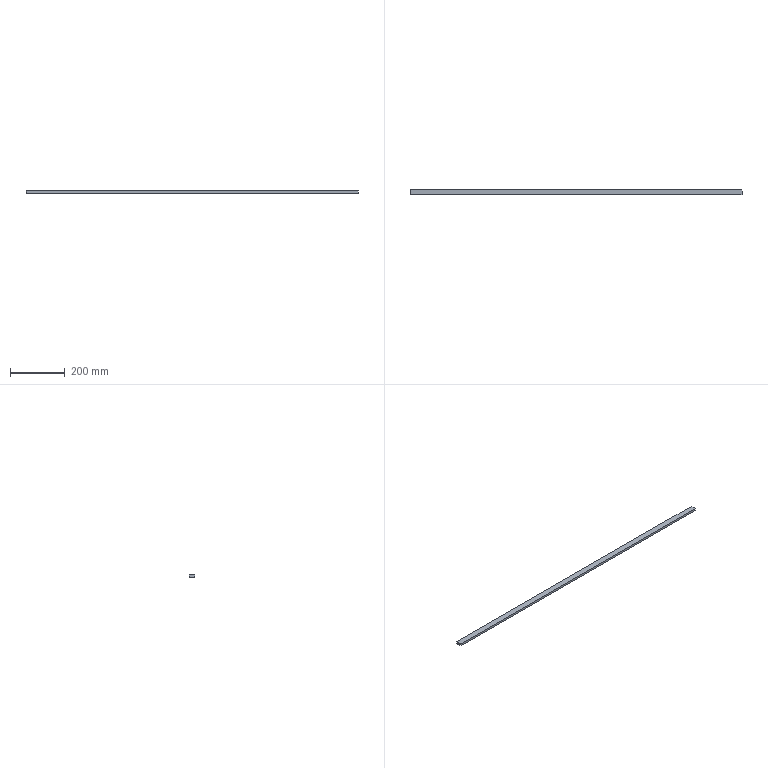Part | SolidWorks | features BaseBody 1 | 1 solid | 9 faces | box 1210 x 20 x 8 mm | volume 193263 mm3 | plane 9
STEP:
#1=CARTESIAN_POINT('',(605.05,-10.,-4.));
#2=VERTEX_POINT('',#1);
#3=CARTESIAN_POINT('',(-602.31,-10.,-4.));
#4=VERTEX_POINT('',#3);
#5=CARTESIAN_POINT('',(1.37,-10.,-4.));
#6=DIRECTION('',(-1.,0.,0.));
#7=VECTOR('',#6,1000.);
#8=LINE('',#5,#7);
#9=EDGE_CURVE('',#2,#4,#8,.T.);
#10=ORIENTED_EDGE('',*,*,#9,.F.);
#11=CARTESIAN_POINT('',(605.05,-10.,4.));
#12=VERTEX_POINT('',#11);
#13=CARTESIAN_POINT('',(605.05,-10.,0.));
#14=DIRECTION('',(0.,0.,-1.));
#15=VECTOR('',#14,1000.);
#16=LINE('',#13,#15);
#17=EDGE_CURVE('',#12,#2,#16,.T.);
#18=ORIENTED_EDGE('',*,*,#17,.F.);
#19=CARTESIAN_POINT('',(-602.31,-10.,4.));
#20=VERTEX_POINT('',#19);
#21=CARTESIAN_POINT('',(1.37,-10.,4.));
#22=DIRECTION('',(1.,0.,0.));
#23=VECTOR('',#22,1000.);
#24=LINE('',#21,#23);
#25=EDGE_CURVE('',#20,#12,#24,.T.);
#26=ORIENTED_EDGE('',*,*,#25,.F.);
#27=CARTESIAN_POINT('',(-602.31,-10.,0.));
#28=DIRECTION('',(0.,0.,1.));
#29=VECTOR('',#28,1000.);
#30=LINE('',#27,#29);
#31=EDGE_CURVE('',#4,#20,#30,.T.);
#32=ORIENTED_EDGE('',*,*,#31,.F.);
#33=EDGE_LOOP('',(#10,#18,#26,#32));
#34=FACE_OUTER_BOUND('',#33,.T.);
#35=CARTESIAN_POINT('',(605.05,-10.,-4.));
#36=DIRECTION('',(0.,1.,0.));
#37=DIRECTION('',(-1.,0.,0.));
#38=AXIS2_PLACEMENT_3D('',#35,#36,#37);
#39=PLANE('',#38);
#40=ADVANCED_FACE('',(#34),#39,.F.);
#41=CARTESIAN_POINT('',(-605.05,10.,4.));
#42=VERTEX_POINT('',#41);
#43=CARTESIAN_POINT('',(-605.05,10.,-4.));
#44=VERTEX_POINT('',#43);
#45=CARTESIAN_POINT('',(-605.05,10.,0.));
#46=DIRECTION('',(0.,0.,-1.));
#47=VECTOR('',#46,1000.);
#48=LINE('',#45,#47);
#49=EDGE_CURVE('',#42,#44,#48,.T.);
#50=ORIENTED_EDGE('',*,*,#49,.T.);
#51=CARTESIAN_POINT('',(-603.68,0.,-4.));
#52=DIRECTION('',(0.1357,-0.9907,0.));
#53=VECTOR('',#52,1000.);
#54=LINE('',#51,#53);
#55=EDGE_CURVE('',#44,#4,#54,.T.);
#56=ORIENTED_EDGE('',*,*,#55,.T.);
#57=ORIENTED_EDGE('',*,*,#31,.T.);
#58=CARTESIAN_POINT('',(-603.68,0.,4.));
#59=DIRECTION('',(-0.1357,0.9907,0.));
#60=VECTOR('',#59,1000.);
#61=LINE('',#58,#60);
#62=EDGE_CURVE('',#20,#42,#61,.T.);
#63=ORIENTED_EDGE('',*,*,#62,.T.);
#64=EDGE_LOOP('',(#50,#56,#57,#63));
#65=FACE_OUTER_BOUND('',#64,.T.);
#66=CARTESIAN_POINT('',(-605.05,10.,-4.));
#67=DIRECTION('',(-0.9907,-0.1357,0.));
#68=DIRECTION('',(0.1357,-0.9907,0.));
#69=AXIS2_PLACEMENT_3D('',#66,#67,#68);
#70=PLANE('',#69);
#71=ADVANCED_FACE('',(#65),#70,.T.);
#72=CARTESIAN_POINT('',(592.561,10.,-4.));
#73=VERTEX_POINT('',#72);
#74=CARTESIAN_POINT('',(592.561,8.975,-4.));
#75=VERTEX_POINT('',#74);
#76=CARTESIAN_POINT('',(592.561,9.488,-4.));
#77=DIRECTION('',(0.,-1.,0.));
#78=VECTOR('',#77,1000.);
#79=LINE('',#76,#78);
#80=EDGE_CURVE('',#73,#75,#79,.T.);
#81=ORIENTED_EDGE('',*,*,#80,.T.);
#82=CARTESIAN_POINT('',(603.97,8.975,-4.));
#83=VERTEX_POINT('',#82);
#84=CARTESIAN_POINT('',(0.,8.975,-4.));
#85=DIRECTION('',(1.,0.,0.));
#86=VECTOR('',#85,1000.);
#87=LINE('',#84,#86);
#88=EDGE_CURVE('',#75,#83,#87,.T.);
#89=ORIENTED_EDGE('',*,*,#88,.T.);
#90=CARTESIAN_POINT('',(605.05,1.773,-4.));
#91=VERTEX_POINT('',#90);
#92=CARTESIAN_POINT('',(603.97,8.975,-4.));
#93=DIRECTION('',(0.1483,-0.9889,0.));
#94=VECTOR('',#93,1000.);
#95=LINE('',#92,#94);
#96=EDGE_CURVE('',#83,#91,#95,.T.);
#97=ORIENTED_EDGE('',*,*,#96,.T.);
#98=CARTESIAN_POINT('',(605.05,0.,-4.));
#99=DIRECTION('',(0.,-1.,0.));
#100=VECTOR('',#99,1000.);
#101=LINE('',#98,#100);
#102=EDGE_CURVE('',#91,#2,#101,.T.);
#103=ORIENTED_EDGE('',*,*,#102,.T.);
#104=ORIENTED_EDGE('',*,*,#9,.T.);
#105=ORIENTED_EDGE('',*,*,#55,.F.);
#106=CARTESIAN_POINT('',(0.,10.,-4.));
#107=DIRECTION('',(1.,0.,0.));
#108=VECTOR('',#107,1000.);
#109=LINE('',#106,#108);
#110=EDGE_CURVE('',#44,#73,#109,.T.);
#111=ORIENTED_EDGE('',*,*,#110,.T.);
#112=EDGE_LOOP('',(#81,#89,#97,#103,#104,#105,#111));
#113=FACE_OUTER_BOUND('',#112,.T.);
#114=CARTESIAN_POINT('',(605.05,-10.,-4.));
#115=DIRECTION('',(0.,0.,-1.));
#116=DIRECTION('',(-1.,0.,0.));
#117=AXIS2_PLACEMENT_3D('',#114,#115,#116);
#118=PLANE('',#117);
#119=ADVANCED_FACE('',(#113),#118,.T.);
#120=CARTESIAN_POINT('',(605.05,1.773,4.));
#121=VERTEX_POINT('',#120);
#122=CARTESIAN_POINT('',(605.05,1.773,0.));
#123=DIRECTION('',(0.,0.,-1.));
#124=VECTOR('',#123,1000.);
#125=LINE('',#122,#124);
#126=EDGE_CURVE('',#121,#91,#125,.T.);
#127=ORIENTED_EDGE('',*,*,#126,.F.);
#128=CARTESIAN_POINT('',(605.05,-4.114,4.));
#129=DIRECTION('',(0.,1.,0.));
#130=VECTOR('',#129,1000.);
#131=LINE('',#128,#130);
#132=EDGE_CURVE('',#12,#121,#131,.T.);
#133=ORIENTED_EDGE('',*,*,#132,.F.);
#134=ORIENTED_EDGE('',*,*,#17,.T.);
#135=ORIENTED_EDGE('',*,*,#102,.F.);
#136=EDGE_LOOP('',(#127,#133,#134,#135));
#137=FACE_OUTER_BOUND('',#136,.T.);
#138=CARTESIAN_POINT('',(605.05,-10.,-4.));
#139=DIRECTION('',(-1.,0.,0.));
#140=DIRECTION('',(0.,0.,1.));
#141=AXIS2_PLACEMENT_3D('',#138,#139,#140);
#142=PLANE('',#141);
#143=ADVANCED_FACE('',(#137),#142,.F.);
#144=CARTESIAN_POINT('',(603.97,8.975,4.));
#145=VERTEX_POINT('',#144);
#146=CARTESIAN_POINT('',(603.97,8.975,4.));
#147=DIRECTION('',(0.1483,-0.9889,0.));
#148=VECTOR('',#147,1000.);
#149=LINE('',#146,#148);
#150=EDGE_CURVE('',#145,#121,#149,.T.);
#151=ORIENTED_EDGE('',*,*,#150,.F.);
#152=CARTESIAN_POINT('',(592.561,8.975,4.));
#153=VERTEX_POINT('',#152);
#154=CARTESIAN_POINT('',(0.,8.975,4.));
#155=DIRECTION('',(1.,0.,0.));
#156=VECTOR('',#155,1000.);
#157=LINE('',#154,#156);
#158=EDGE_CURVE('',#153,#145,#157,.T.);
#159=ORIENTED_EDGE('',*,*,#158,.F.);
#160=CARTESIAN_POINT('',(592.561,10.,4.));
#161=VERTEX_POINT('',#160);
#162=CARTESIAN_POINT('',(592.561,9.488,4.));
#163=DIRECTION('',(0.,1.,0.));
#164=VECTOR('',#163,1000.);
#165=LINE('',#162,#164);
#166=EDGE_CURVE('',#153,#161,#165,.T.);
#167=ORIENTED_EDGE('',*,*,#166,.T.);
#168=CARTESIAN_POINT('',(0.,10.,4.));
#169=DIRECTION('',(1.,0.,0.));
#170=VECTOR('',#169,1000.);
#171=LINE('',#168,#170);
#172=EDGE_CURVE('',#42,#161,#171,.T.);
#173=ORIENTED_EDGE('',*,*,#172,.F.);
#174=ORIENTED_EDGE('',*,*,#62,.F.);
#175=ORIENTED_EDGE('',*,*,#25,.T.);
#176=ORIENTED_EDGE('',*,*,#132,.T.);
#177=EDGE_LOOP('',(#151,#159,#167,#173,#174,#175,#176));
#178=FACE_OUTER_BOUND('',#177,.T.);
#179=CARTESIAN_POINT('',(605.05,-10.,4.));
#180=DIRECTION('',(0.,0.,-1.));
#181=DIRECTION('',(-1.,0.,0.));
#182=AXIS2_PLACEMENT_3D('',#179,#180,#181);
#183=PLANE('',#182);
#184=ADVANCED_FACE('',(#178),#183,.F.);
#185=CARTESIAN_POINT('',(592.561,10.,0.));
#186=DIRECTION('',(0.,0.,1.));
#187=VECTOR('',#186,1000.);
#188=LINE('',#185,#187);
#189=EDGE_CURVE('',#73,#161,#188,.T.);
#190=ORIENTED_EDGE('',*,*,#189,.F.);
#191=ORIENTED_EDGE('',*,*,#110,.F.);
#192=ORIENTED_EDGE('',*,*,#49,.F.);
#193=ORIENTED_EDGE('',*,*,#172,.T.);
#194=EDGE_LOOP('',(#190,#191,#192,#193));
#195=FACE_OUTER_BOUND('',#194,.T.);
#196=CARTESIAN_POINT('',(-605.05,10.,-4.));
#197=DIRECTION('',(0.,-1.,0.));
#198=DIRECTION('',(1.,0.,0.));
#199=AXIS2_PLACEMENT_3D('',#196,#197,#198);
#200=PLANE('',#199);
#201=ADVANCED_FACE('',(#195),#200,.F.);
#202=ORIENTED_EDGE('',*,*,#88,.F.);
#203=CARTESIAN_POINT('',(592.561,8.975,0.));
#204=DIRECTION('',(0.,0.,-1.));
#205=VECTOR('',#204,1000.);
#206=LINE('',#203,#205);
#207=EDGE_CURVE('',#153,#75,#206,.T.);
#208=ORIENTED_EDGE('',*,*,#207,.F.);
#209=ORIENTED_EDGE('',*,*,#158,.T.);
#210=CARTESIAN_POINT('',(603.97,8.975,0.));
#211=DIRECTION('',(0.,0.,1.));
#212=VECTOR('',#211,1000.);
#213=LINE('',#210,#212);
#214=EDGE_CURVE('',#83,#145,#213,.T.);
#215=ORIENTED_EDGE('',*,*,#214,.F.);
#216=EDGE_LOOP('',(#202,#208,#209,#215));
#217=FACE_OUTER_BOUND('',#216,.T.);
#218=CARTESIAN_POINT('',(592.561,8.975,4.));
#219=DIRECTION('',(0.,-1.,0.));
#220=DIRECTION('',(0.,0.,-1.));
#221=AXIS2_PLACEMENT_3D('',#218,#219,#220);
#222=PLANE('',#221);
#223=ADVANCED_FACE('',(#217),#222,.F.);
#224=ORIENTED_EDGE('',*,*,#96,.F.);
#225=ORIENTED_EDGE('',*,*,#214,.T.);
#226=ORIENTED_EDGE('',*,*,#150,.T.);
#227=ORIENTED_EDGE('',*,*,#126,.T.);
#228=EDGE_LOOP('',(#224,#225,#226,#227));
#229=FACE_OUTER_BOUND('',#228,.T.);
#230=CARTESIAN_POINT('',(603.97,8.975,-4.));
#231=DIRECTION('',(-0.9889,-0.1483,0.));
#232=DIRECTION('',(0.1483,-0.9889,0.));
#233=AXIS2_PLACEMENT_3D('',#230,#231,#232);
#234=PLANE('',#233);
#235=ADVANCED_FACE('',(#229),#234,.F.);
#236=ORIENTED_EDGE('',*,*,#80,.F.);
#237=ORIENTED_EDGE('',*,*,#189,.T.);
#238=ORIENTED_EDGE('',*,*,#166,.F.);
#239=ORIENTED_EDGE('',*,*,#207,.T.);
#240=EDGE_LOOP('',(#236,#237,#238,#239));
#241=FACE_OUTER_BOUND('',#240,.T.);
#242=CARTESIAN_POINT('',(592.561,8.975,-4.));
#243=DIRECTION('',(-1.,0.,0.));
#244=DIRECTION('',(0.,0.,1.));
#245=AXIS2_PLACEMENT_3D('',#242,#243,#244);
#246=PLANE('',#245);
#247=ADVANCED_FACE('',(#241),#246,.F.);
#248=CLOSED_SHELL('',(#40,#71,#119,#143,#184,#201,#223,#235,#247));
#249=MANIFOLD_SOLID_BREP('',#248);
#250=CARTESIAN_POINT('',(0.,0.,0.));
#251=DIRECTION('',(0.,0.,1.));
#252=DIRECTION('',(1.,0.,0.));
#253=AXIS2_PLACEMENT_3D('',#250,#251,#252);
#254=(LENGTH_UNIT()NAMED_UNIT(*)SI_UNIT(.MILLI.,.METRE.));
#255=UNCERTAINTY_MEASURE_WITH_UNIT(LENGTH_MEASURE(0.00001),#254,'','');
#256=(NAMED_UNIT(*)PLANE_ANGLE_UNIT()SI_UNIT($,.RADIAN.));
#257=(NAMED_UNIT(*)SI_UNIT($,.STERADIAN.)SOLID_ANGLE_UNIT());
#258=(GEOMETRIC_REPRESENTATION_CONTEXT(3)GLOBAL_UNCERTAINTY_ASSIGNED_CONTEXT((#255))GLOBAL_UNIT_ASSIGNED_CONTEXT((#254,#256,#257))REPRESENTATION_CONTEXT('',''));
#259=ADVANCED_BREP_SHAPE_REPRESENTATION('',(#249,#253),#258);